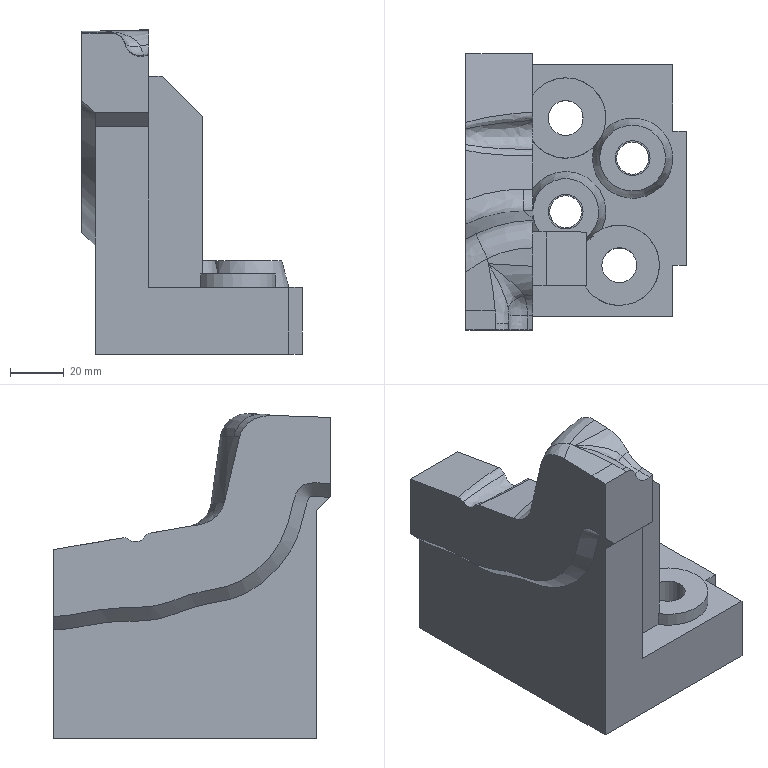Part | NX | features solid 2 | 1 solid | 61 faces | box 82.317 x 103.162 x 121.233 mm | volume 359413 mm3 | plane 26 | spline 23 | cylinder 9 | cone 3 | commonest cylinder face diameters 13 x4 30 x3 12 x2